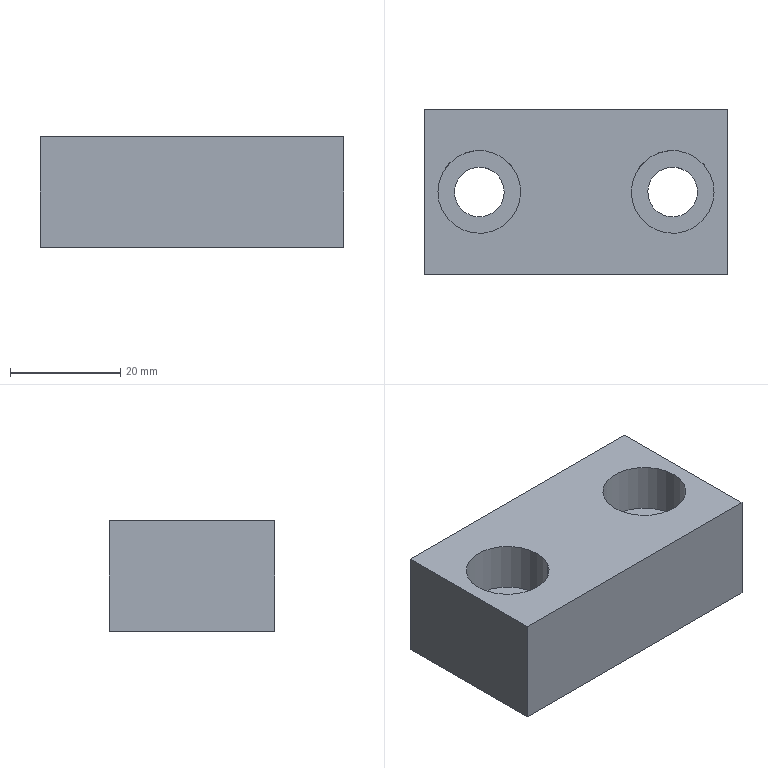Part | CATIA | 1 solid | 16 faces | box 55 x 30 x 20 mm | volume 28420 mm3 | plane 8 | cylinder 8 | commonest cylinder face diameters 9 x4 15 x4
STEP:
#1=CARTESIAN_POINT('',(27.5,15.,0.));
#2=VERTEX_POINT('',#1);
#3=CARTESIAN_POINT('',(27.5,15.,20.));
#4=VERTEX_POINT('',#3);
#5=CARTESIAN_POINT('',(27.5,15.,10.));
#6=DIRECTION('',(0.,0.,1.));
#7=VECTOR('',#6,1.);
#8=LINE('',#5,#7);
#9=EDGE_CURVE('',#2,#4,#8,.T.);
#10=ORIENTED_EDGE('',*,*,#9,.F.);
#11=CARTESIAN_POINT('',(-27.5,15.,0.));
#12=VERTEX_POINT('',#11);
#13=CARTESIAN_POINT('',(0.,15.,0.));
#14=DIRECTION('',(1.,0.,0.));
#15=VECTOR('',#14,1.);
#16=LINE('',#13,#15);
#17=EDGE_CURVE('',#2,#12,#16,.F.);
#18=ORIENTED_EDGE('',*,*,#17,.T.);
#19=CARTESIAN_POINT('',(-27.5,15.,20.));
#20=VERTEX_POINT('',#19);
#21=CARTESIAN_POINT('',(-27.5,15.,10.));
#22=DIRECTION('',(0.,0.,1.));
#23=VECTOR('',#22,1.);
#24=LINE('',#21,#23);
#25=EDGE_CURVE('',#12,#20,#24,.T.);
#26=ORIENTED_EDGE('',*,*,#25,.T.);
#27=CARTESIAN_POINT('',(0.,15.,20.));
#28=DIRECTION('',(1.,0.,0.));
#29=VECTOR('',#28,1.);
#30=LINE('',#27,#29);
#31=EDGE_CURVE('',#4,#20,#30,.F.);
#32=ORIENTED_EDGE('',*,*,#31,.F.);
#33=EDGE_LOOP('',(#10,#18,#26,#32));
#34=FACE_OUTER_BOUND('',#33,.T.);
#35=CARTESIAN_POINT('',(-27.5,15.,0.));
#36=DIRECTION('',(0.,-1.,0.));
#37=DIRECTION('',(1.,0.,0.));
#38=AXIS2_PLACEMENT_3D('',#35,#36,#37);
#39=PLANE('',#38);
#40=ADVANCED_FACE('',(#34),#39,.F.);
#41=ORIENTED_EDGE('',*,*,#25,.F.);
#42=CARTESIAN_POINT('',(-27.5,-15.,0.));
#43=VERTEX_POINT('',#42);
#44=CARTESIAN_POINT('',(-27.5,0.,0.));
#45=DIRECTION('',(0.,1.,0.));
#46=VECTOR('',#45,1.);
#47=LINE('',#44,#46);
#48=EDGE_CURVE('',#12,#43,#47,.F.);
#49=ORIENTED_EDGE('',*,*,#48,.T.);
#50=CARTESIAN_POINT('',(-27.5,-15.,20.));
#51=VERTEX_POINT('',#50);
#52=CARTESIAN_POINT('',(-27.5,-15.,10.));
#53=DIRECTION('',(0.,0.,1.));
#54=VECTOR('',#53,1.);
#55=LINE('',#52,#54);
#56=EDGE_CURVE('',#43,#51,#55,.T.);
#57=ORIENTED_EDGE('',*,*,#56,.T.);
#58=CARTESIAN_POINT('',(-27.5,0.,20.));
#59=DIRECTION('',(0.,1.,0.));
#60=VECTOR('',#59,1.);
#61=LINE('',#58,#60);
#62=EDGE_CURVE('',#20,#51,#61,.F.);
#63=ORIENTED_EDGE('',*,*,#62,.F.);
#64=EDGE_LOOP('',(#41,#49,#57,#63));
#65=FACE_OUTER_BOUND('',#64,.T.);
#66=CARTESIAN_POINT('',(-27.5,-15.,0.));
#67=DIRECTION('',(1.,0.,0.));
#68=DIRECTION('',(0.,1.,0.));
#69=AXIS2_PLACEMENT_3D('',#66,#67,#68);
#70=PLANE('',#69);
#71=ADVANCED_FACE('',(#65),#70,.F.);
#72=ORIENTED_EDGE('',*,*,#56,.F.);
#73=CARTESIAN_POINT('',(27.5,-15.,0.));
#74=VERTEX_POINT('',#73);
#75=CARTESIAN_POINT('',(0.,-15.,0.));
#76=DIRECTION('',(-1.,0.,0.));
#77=VECTOR('',#76,1.);
#78=LINE('',#75,#77);
#79=EDGE_CURVE('',#43,#74,#78,.F.);
#80=ORIENTED_EDGE('',*,*,#79,.T.);
#81=CARTESIAN_POINT('',(27.5,-15.,20.));
#82=VERTEX_POINT('',#81);
#83=CARTESIAN_POINT('',(27.5,-15.,10.));
#84=DIRECTION('',(0.,0.,1.));
#85=VECTOR('',#84,1.);
#86=LINE('',#83,#85);
#87=EDGE_CURVE('',#74,#82,#86,.T.);
#88=ORIENTED_EDGE('',*,*,#87,.T.);
#89=CARTESIAN_POINT('',(0.,-15.,20.));
#90=DIRECTION('',(-1.,0.,0.));
#91=VECTOR('',#90,1.);
#92=LINE('',#89,#91);
#93=EDGE_CURVE('',#51,#82,#92,.F.);
#94=ORIENTED_EDGE('',*,*,#93,.F.);
#95=EDGE_LOOP('',(#72,#80,#88,#94));
#96=FACE_OUTER_BOUND('',#95,.T.);
#97=CARTESIAN_POINT('',(27.5,-15.,0.));
#98=DIRECTION('',(0.,1.,0.));
#99=DIRECTION('',(-1.,0.,0.));
#100=AXIS2_PLACEMENT_3D('',#97,#98,#99);
#101=PLANE('',#100);
#102=ADVANCED_FACE('',(#96),#101,.F.);
#103=ORIENTED_EDGE('',*,*,#87,.F.);
#104=CARTESIAN_POINT('',(27.5,0.,0.));
#105=DIRECTION('',(0.,-1.,0.));
#106=VECTOR('',#105,1.);
#107=LINE('',#104,#106);
#108=EDGE_CURVE('',#74,#2,#107,.F.);
#109=ORIENTED_EDGE('',*,*,#108,.T.);
#110=ORIENTED_EDGE('',*,*,#9,.T.);
#111=CARTESIAN_POINT('',(27.5,0.,20.));
#112=DIRECTION('',(0.,-1.,0.));
#113=VECTOR('',#112,1.);
#114=LINE('',#111,#113);
#115=EDGE_CURVE('',#82,#4,#114,.F.);
#116=ORIENTED_EDGE('',*,*,#115,.F.);
#117=EDGE_LOOP('',(#103,#109,#110,#116));
#118=FACE_OUTER_BOUND('',#117,.T.);
#119=CARTESIAN_POINT('',(27.5,15.,0.));
#120=DIRECTION('',(-1.,0.,0.));
#121=DIRECTION('',(0.,-1.,0.));
#122=AXIS2_PLACEMENT_3D('',#119,#120,#121);
#123=PLANE('',#122);
#124=ADVANCED_FACE('',(#118),#123,.F.);
#125=ORIENTED_EDGE('',*,*,#31,.T.);
#126=ORIENTED_EDGE('',*,*,#62,.T.);
#127=ORIENTED_EDGE('',*,*,#93,.T.);
#128=ORIENTED_EDGE('',*,*,#115,.T.);
#129=EDGE_LOOP('',(#125,#126,#127,#128));
#130=FACE_OUTER_BOUND('',#129,.T.);
#131=CARTESIAN_POINT('',(-10.918,-3.596,20.));
#132=VERTEX_POINT('',#131);
#133=CARTESIAN_POINT('',(-24.082,3.596,20.));
#134=VERTEX_POINT('',#133);
#135=CARTESIAN_POINT('',(-17.5,0.,20.));
#136=DIRECTION('',(0.,0.,1.));
#137=AXIS2_PLACEMENT_3D('',#135,#136,$);
#138=CIRCLE('',#137,7.5);
#139=EDGE_CURVE('',#132,#134,#138,.T.);
#140=ORIENTED_EDGE('',*,*,#139,.F.);
#141=CARTESIAN_POINT('',(-17.5,0.,20.));
#142=DIRECTION('',(0.,0.,1.));
#143=AXIS2_PLACEMENT_3D('',#141,#142,$);
#144=CIRCLE('',#143,7.5);
#145=EDGE_CURVE('',#134,#132,#144,.T.);
#146=ORIENTED_EDGE('',*,*,#145,.F.);
#147=EDGE_LOOP('',(#140,#146));
#148=FACE_BOUND('',#147,.T.);
#149=CARTESIAN_POINT('',(24.082,-3.596,20.));
#150=VERTEX_POINT('',#149);
#151=CARTESIAN_POINT('',(10.918,3.596,20.));
#152=VERTEX_POINT('',#151);
#153=CARTESIAN_POINT('',(17.5,0.,20.));
#154=DIRECTION('',(0.,0.,1.));
#155=AXIS2_PLACEMENT_3D('',#153,#154,$);
#156=CIRCLE('',#155,7.5);
#157=EDGE_CURVE('',#150,#152,#156,.T.);
#158=ORIENTED_EDGE('',*,*,#157,.F.);
#159=CARTESIAN_POINT('',(17.5,0.,20.));
#160=DIRECTION('',(0.,0.,1.));
#161=AXIS2_PLACEMENT_3D('',#159,#160,$);
#162=CIRCLE('',#161,7.5);
#163=EDGE_CURVE('',#152,#150,#162,.T.);
#164=ORIENTED_EDGE('',*,*,#163,.F.);
#165=EDGE_LOOP('',(#158,#164));
#166=FACE_BOUND('',#165,.T.);
#167=CARTESIAN_POINT('',(0.,0.,20.));
#168=DIRECTION('',(0.,0.,1.));
#169=DIRECTION('',(1.,0.,0.));
#170=AXIS2_PLACEMENT_3D('',#167,#168,#169);
#171=PLANE('',#170);
#172=ADVANCED_FACE('',(#130,#148,#166),#171,.T.);
#173=ORIENTED_EDGE('',*,*,#108,.F.);
#174=ORIENTED_EDGE('',*,*,#79,.F.);
#175=ORIENTED_EDGE('',*,*,#48,.F.);
#176=ORIENTED_EDGE('',*,*,#17,.F.);
#177=EDGE_LOOP('',(#173,#174,#175,#176));
#178=FACE_OUTER_BOUND('',#177,.T.);
#179=CARTESIAN_POINT('',(-21.449,2.157,0.));
#180=VERTEX_POINT('',#179);
#181=CARTESIAN_POINT('',(-13.551,-2.157,0.));
#182=VERTEX_POINT('',#181);
#183=CARTESIAN_POINT('',(-17.5,0.,0.));
#184=DIRECTION('',(0.,0.,1.));
#185=AXIS2_PLACEMENT_3D('',#183,#184,$);
#186=CIRCLE('',#185,4.5);
#187=EDGE_CURVE('',#180,#182,#186,.T.);
#188=ORIENTED_EDGE('',*,*,#187,.T.);
#189=CARTESIAN_POINT('',(-17.5,0.,0.));
#190=DIRECTION('',(0.,0.,1.));
#191=AXIS2_PLACEMENT_3D('',#189,#190,$);
#192=CIRCLE('',#191,4.5);
#193=EDGE_CURVE('',#182,#180,#192,.T.);
#194=ORIENTED_EDGE('',*,*,#193,.T.);
#195=EDGE_LOOP('',(#188,#194));
#196=FACE_BOUND('',#195,.T.);
#197=CARTESIAN_POINT('',(13.551,2.157,0.));
#198=VERTEX_POINT('',#197);
#199=CARTESIAN_POINT('',(21.449,-2.157,0.));
#200=VERTEX_POINT('',#199);
#201=CARTESIAN_POINT('',(17.5,0.,0.));
#202=DIRECTION('',(0.,0.,1.));
#203=AXIS2_PLACEMENT_3D('',#201,#202,$);
#204=CIRCLE('',#203,4.5);
#205=EDGE_CURVE('',#198,#200,#204,.T.);
#206=ORIENTED_EDGE('',*,*,#205,.T.);
#207=CARTESIAN_POINT('',(17.5,0.,0.));
#208=DIRECTION('',(0.,0.,1.));
#209=AXIS2_PLACEMENT_3D('',#207,#208,$);
#210=CIRCLE('',#209,4.5);
#211=EDGE_CURVE('',#200,#198,#210,.T.);
#212=ORIENTED_EDGE('',*,*,#211,.T.);
#213=EDGE_LOOP('',(#206,#212));
#214=FACE_BOUND('',#213,.T.);
#215=CARTESIAN_POINT('',(0.,0.,0.));
#216=DIRECTION('',(0.,0.,1.));
#217=DIRECTION('',(1.,0.,0.));
#218=AXIS2_PLACEMENT_3D('',#215,#216,#217);
#219=PLANE('',#218);
#220=ADVANCED_FACE('',(#178,#196,#214),#219,.F.);
#221=CARTESIAN_POINT('',(24.082,-3.596,11.));
#222=VERTEX_POINT('',#221);
#223=CARTESIAN_POINT('',(10.918,3.596,11.));
#224=VERTEX_POINT('',#223);
#225=CARTESIAN_POINT('',(17.5,0.,11.));
#226=DIRECTION('',(0.,0.,-1.));
#227=AXIS2_PLACEMENT_3D('',#225,#226,$);
#228=CIRCLE('',#227,7.5);
#229=EDGE_CURVE('',#222,#224,#228,.T.);
#230=ORIENTED_EDGE('',*,*,#229,.F.);
#231=CARTESIAN_POINT('',(17.5,0.,11.));
#232=DIRECTION('',(0.,0.,-1.));
#233=AXIS2_PLACEMENT_3D('',#231,#232,$);
#234=CIRCLE('',#233,7.5);
#235=EDGE_CURVE('',#224,#222,#234,.T.);
#236=ORIENTED_EDGE('',*,*,#235,.F.);
#237=EDGE_LOOP('',(#230,#236));
#238=FACE_OUTER_BOUND('',#237,.T.);
#239=CARTESIAN_POINT('',(13.551,2.157,11.));
#240=VERTEX_POINT('',#239);
#241=CARTESIAN_POINT('',(21.449,-2.157,11.));
#242=VERTEX_POINT('',#241);
#243=CARTESIAN_POINT('',(17.5,0.,11.));
#244=DIRECTION('',(0.,0.,-1.));
#245=AXIS2_PLACEMENT_3D('',#243,#244,$);
#246=CIRCLE('',#245,4.5);
#247=EDGE_CURVE('',#240,#242,#246,.T.);
#248=ORIENTED_EDGE('',*,*,#247,.T.);
#249=CARTESIAN_POINT('',(17.5,0.,11.));
#250=DIRECTION('',(0.,0.,-1.));
#251=AXIS2_PLACEMENT_3D('',#249,#250,$);
#252=CIRCLE('',#251,4.5);
#253=EDGE_CURVE('',#242,#240,#252,.T.);
#254=ORIENTED_EDGE('',*,*,#253,.T.);
#255=EDGE_LOOP('',(#248,#254));
#256=FACE_BOUND('',#255,.T.);
#257=CARTESIAN_POINT('',(-13.,0.,11.));
#258=DIRECTION('',(0.,0.,-1.));
#259=DIRECTION('',(1.,0.,0.));
#260=AXIS2_PLACEMENT_3D('',#257,#258,#259);
#261=PLANE('',#260);
#262=ADVANCED_FACE('',(#238,#256),#261,.F.);
#263=ORIENTED_EDGE('',*,*,#157,.T.);
#264=CARTESIAN_POINT('',(10.918,3.596,15.7));
#265=DIRECTION('',(0.,0.,-1.));
#266=VECTOR('',#265,1.);
#267=LINE('',#264,#266);
#268=EDGE_CURVE('',#224,#152,#267,.F.);
#269=ORIENTED_EDGE('',*,*,#268,.F.);
#270=ORIENTED_EDGE('',*,*,#235,.T.);
#271=CARTESIAN_POINT('',(24.082,-3.596,15.7));
#272=DIRECTION('',(0.,0.,-1.));
#273=VECTOR('',#272,1.);
#274=LINE('',#271,#273);
#275=EDGE_CURVE('',#222,#150,#274,.F.);
#276=ORIENTED_EDGE('',*,*,#275,.T.);
#277=EDGE_LOOP('',(#263,#269,#270,#276));
#278=FACE_OUTER_BOUND('',#277,.T.);
#279=CARTESIAN_POINT('',(17.5,0.,19.9));
#280=DIRECTION('',(0.,0.,-1.));
#281=DIRECTION('',(0.8776,-0.4794,0.));
#282=AXIS2_PLACEMENT_3D('',#279,#280,#281);
#283=CYLINDRICAL_SURFACE('',#282,7.5);
#284=ADVANCED_FACE('',(#278),#283,.F.);
#285=ORIENTED_EDGE('',*,*,#163,.T.);
#286=ORIENTED_EDGE('',*,*,#275,.F.);
#287=ORIENTED_EDGE('',*,*,#229,.T.);
#288=ORIENTED_EDGE('',*,*,#268,.T.);
#289=EDGE_LOOP('',(#285,#286,#287,#288));
#290=FACE_OUTER_BOUND('',#289,.T.);
#291=ADVANCED_FACE('',(#290),#283,.F.);
#292=ORIENTED_EDGE('',*,*,#205,.F.);
#293=CARTESIAN_POINT('',(13.551,2.157,5.3));
#294=DIRECTION('',(0.,0.,-1.));
#295=VECTOR('',#294,1.);
#296=LINE('',#293,#295);
#297=EDGE_CURVE('',#198,#240,#296,.F.);
#298=ORIENTED_EDGE('',*,*,#297,.T.);
#299=ORIENTED_EDGE('',*,*,#253,.F.);
#300=CARTESIAN_POINT('',(21.449,-2.157,5.3));
#301=DIRECTION('',(0.,0.,-1.));
#302=VECTOR('',#301,1.);
#303=LINE('',#300,#302);
#304=EDGE_CURVE('',#200,#242,#303,.F.);
#305=ORIENTED_EDGE('',*,*,#304,.F.);
#306=EDGE_LOOP('',(#292,#298,#299,#305));
#307=FACE_OUTER_BOUND('',#306,.T.);
#308=CARTESIAN_POINT('',(17.5,0.,19.9));
#309=DIRECTION('',(0.,0.,-1.));
#310=DIRECTION('',(0.8776,-0.4794,0.));
#311=AXIS2_PLACEMENT_3D('',#308,#309,#310);
#312=CYLINDRICAL_SURFACE('',#311,4.5);
#313=ADVANCED_FACE('',(#307),#312,.F.);
#314=ORIENTED_EDGE('',*,*,#211,.F.);
#315=ORIENTED_EDGE('',*,*,#304,.T.);
#316=ORIENTED_EDGE('',*,*,#247,.F.);
#317=ORIENTED_EDGE('',*,*,#297,.F.);
#318=EDGE_LOOP('',(#314,#315,#316,#317));
#319=FACE_OUTER_BOUND('',#318,.T.);
#320=ADVANCED_FACE('',(#319),#312,.F.);
#321=CARTESIAN_POINT('',(-10.918,-3.596,11.));
#322=VERTEX_POINT('',#321);
#323=CARTESIAN_POINT('',(-24.082,3.596,11.));
#324=VERTEX_POINT('',#323);
#325=CARTESIAN_POINT('',(-17.5,0.,11.));
#326=DIRECTION('',(0.,0.,-1.));
#327=AXIS2_PLACEMENT_3D('',#325,#326,$);
#328=CIRCLE('',#327,7.5);
#329=EDGE_CURVE('',#322,#324,#328,.T.);
#330=ORIENTED_EDGE('',*,*,#329,.F.);
#331=CARTESIAN_POINT('',(-17.5,0.,11.));
#332=DIRECTION('',(0.,0.,-1.));
#333=AXIS2_PLACEMENT_3D('',#331,#332,$);
#334=CIRCLE('',#333,7.5);
#335=EDGE_CURVE('',#324,#322,#334,.T.);
#336=ORIENTED_EDGE('',*,*,#335,.F.);
#337=EDGE_LOOP('',(#330,#336));
#338=FACE_OUTER_BOUND('',#337,.T.);
#339=CARTESIAN_POINT('',(-21.449,2.157,11.));
#340=VERTEX_POINT('',#339);
#341=CARTESIAN_POINT('',(-13.551,-2.157,11.));
#342=VERTEX_POINT('',#341);
#343=CARTESIAN_POINT('',(-17.5,0.,11.));
#344=DIRECTION('',(0.,0.,-1.));
#345=AXIS2_PLACEMENT_3D('',#343,#344,$);
#346=CIRCLE('',#345,4.5);
#347=EDGE_CURVE('',#340,#342,#346,.T.);
#348=ORIENTED_EDGE('',*,*,#347,.T.);
#349=CARTESIAN_POINT('',(-17.5,0.,11.));
#350=DIRECTION('',(0.,0.,-1.));
#351=AXIS2_PLACEMENT_3D('',#349,#350,$);
#352=CIRCLE('',#351,4.5);
#353=EDGE_CURVE('',#342,#340,#352,.T.);
#354=ORIENTED_EDGE('',*,*,#353,.T.);
#355=EDGE_LOOP('',(#348,#354));
#356=FACE_BOUND('',#355,.T.);
#357=ADVANCED_FACE('',(#338,#356),#261,.F.);
#358=ORIENTED_EDGE('',*,*,#139,.T.);
#359=CARTESIAN_POINT('',(-24.082,3.596,15.7));
#360=DIRECTION('',(0.,0.,-1.));
#361=VECTOR('',#360,1.);
#362=LINE('',#359,#361);
#363=EDGE_CURVE('',#324,#134,#362,.F.);
#364=ORIENTED_EDGE('',*,*,#363,.F.);
#365=ORIENTED_EDGE('',*,*,#335,.T.);
#366=CARTESIAN_POINT('',(-10.918,-3.596,15.7));
#367=DIRECTION('',(0.,0.,-1.));
#368=VECTOR('',#367,1.);
#369=LINE('',#366,#368);
#370=EDGE_CURVE('',#322,#132,#369,.F.);
#371=ORIENTED_EDGE('',*,*,#370,.T.);
#372=EDGE_LOOP('',(#358,#364,#365,#371));
#373=FACE_OUTER_BOUND('',#372,.T.);
#374=CARTESIAN_POINT('',(-17.5,0.,19.9));
#375=DIRECTION('',(0.,0.,-1.));
#376=DIRECTION('',(0.8776,-0.4794,0.));
#377=AXIS2_PLACEMENT_3D('',#374,#375,#376);
#378=CYLINDRICAL_SURFACE('',#377,7.5);
#379=ADVANCED_FACE('',(#373),#378,.F.);
#380=ORIENTED_EDGE('',*,*,#145,.T.);
#381=ORIENTED_EDGE('',*,*,#370,.F.);
#382=ORIENTED_EDGE('',*,*,#329,.T.);
#383=ORIENTED_EDGE('',*,*,#363,.T.);
#384=EDGE_LOOP('',(#380,#381,#382,#383));
#385=FACE_OUTER_BOUND('',#384,.T.);
#386=ADVANCED_FACE('',(#385),#378,.F.);
#387=ORIENTED_EDGE('',*,*,#187,.F.);
#388=CARTESIAN_POINT('',(-21.449,2.157,5.3));
#389=DIRECTION('',(0.,0.,-1.));
#390=VECTOR('',#389,1.);
#391=LINE('',#388,#390);
#392=EDGE_CURVE('',#180,#340,#391,.F.);
#393=ORIENTED_EDGE('',*,*,#392,.T.);
#394=ORIENTED_EDGE('',*,*,#353,.F.);
#395=CARTESIAN_POINT('',(-13.551,-2.157,5.3));
#396=DIRECTION('',(0.,0.,-1.));
#397=VECTOR('',#396,1.);
#398=LINE('',#395,#397);
#399=EDGE_CURVE('',#182,#342,#398,.F.);
#400=ORIENTED_EDGE('',*,*,#399,.F.);
#401=EDGE_LOOP('',(#387,#393,#394,#400));
#402=FACE_OUTER_BOUND('',#401,.T.);
#403=CARTESIAN_POINT('',(-17.5,0.,19.9));
#404=DIRECTION('',(0.,0.,-1.));
#405=DIRECTION('',(0.8776,-0.4794,0.));
#406=AXIS2_PLACEMENT_3D('',#403,#404,#405);
#407=CYLINDRICAL_SURFACE('',#406,4.5);
#408=ADVANCED_FACE('',(#402),#407,.F.);
#409=ORIENTED_EDGE('',*,*,#193,.F.);
#410=ORIENTED_EDGE('',*,*,#399,.T.);
#411=ORIENTED_EDGE('',*,*,#347,.F.);
#412=ORIENTED_EDGE('',*,*,#392,.F.);
#413=EDGE_LOOP('',(#409,#410,#411,#412));
#414=FACE_OUTER_BOUND('',#413,.T.);
#415=ADVANCED_FACE('',(#414),#407,.F.);
#416=CLOSED_SHELL('',(#40,#71,#102,#124,#172,#220,#262,#284,#291,#313,#320,#357,#379,#386,#408,#415));
#417=MANIFOLD_SOLID_BREP('',#416);
#418=(LENGTH_UNIT()NAMED_UNIT(*)SI_UNIT(.MILLI.,.METRE.));
#419=UNCERTAINTY_MEASURE_WITH_UNIT(LENGTH_MEASURE(0.005),#418,'','');
#420=(NAMED_UNIT(*)PLANE_ANGLE_UNIT()SI_UNIT($,.RADIAN.));
#421=(NAMED_UNIT(*)SI_UNIT($,.STERADIAN.)SOLID_ANGLE_UNIT());
#422=(GEOMETRIC_REPRESENTATION_CONTEXT(3)GLOBAL_UNCERTAINTY_ASSIGNED_CONTEXT((#419))GLOBAL_UNIT_ASSIGNED_CONTEXT((#418,#420,#421))REPRESENTATION_CONTEXT('',''));
#423=ADVANCED_BREP_SHAPE_REPRESENTATION('',(#417),#422);